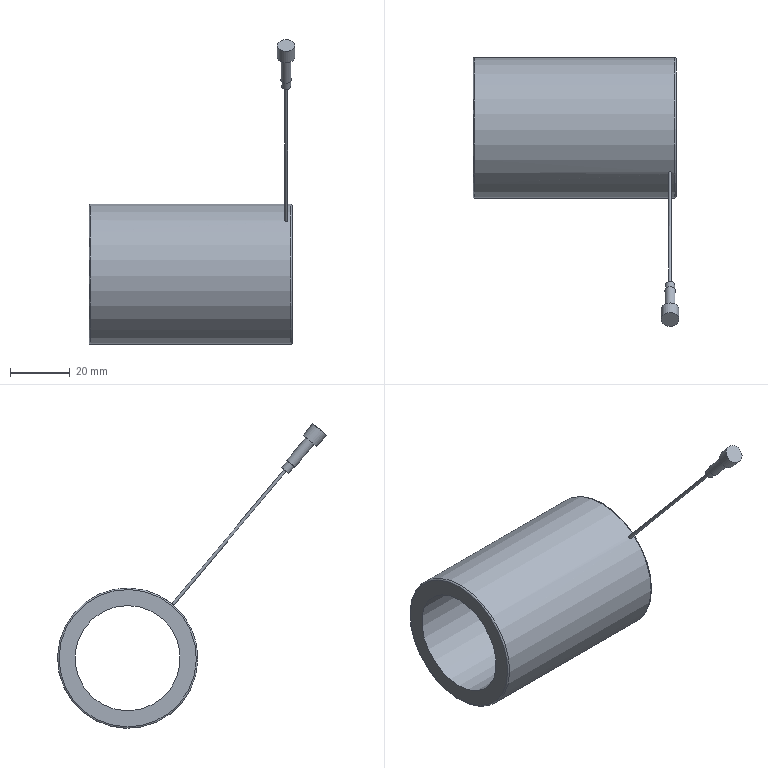Part | STEP file | Tube Heater_Bala35_toe-2 | 1 solid | 14 faces | box 69 x 90.077 x 102.033 mm | volume 51909 mm3 | cylinder 6 | plane 6 | torus 2 | commonest cylinder face diameters 1 x1 3 x1 3.6 x1 6 x1 35.25 x1 47 x1